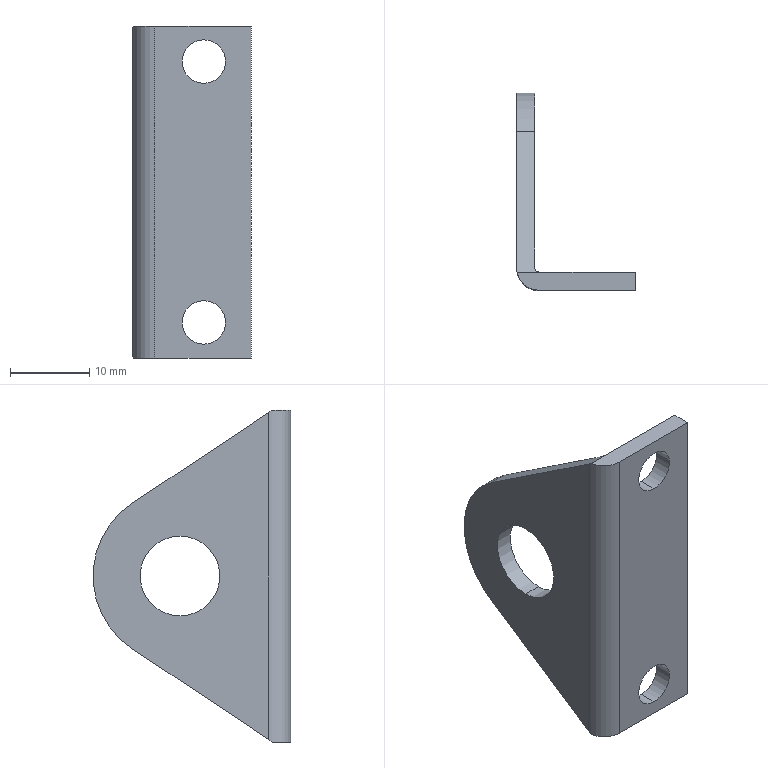Part | STEP file | QA-HI_SBA-16-LB_(150) | 1 solid | 18 faces | box 15 x 25 x 42 mm | volume 2467 mm3 | cylinder 9 | plane 9 | commonest cylinder face diameters 5.5 x4 10.1 x2 1 x1 5.6 x1 22 x1